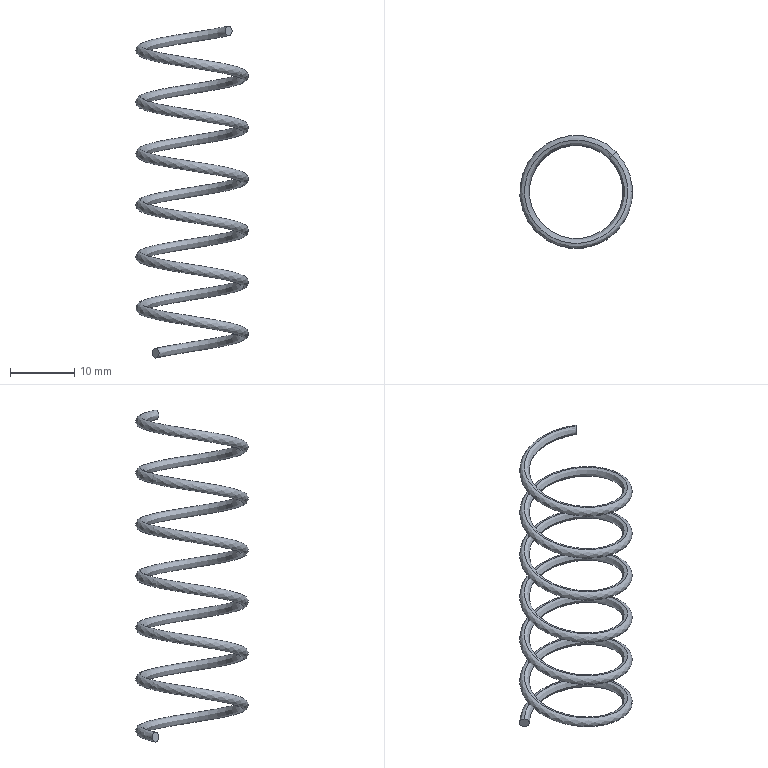Part | STEP file | Spring A | 1 solid | 4 faces | box 17.5 x 17.5 x 51.5 mm | volume 555.182 mm3 | spline 2 | plane 2